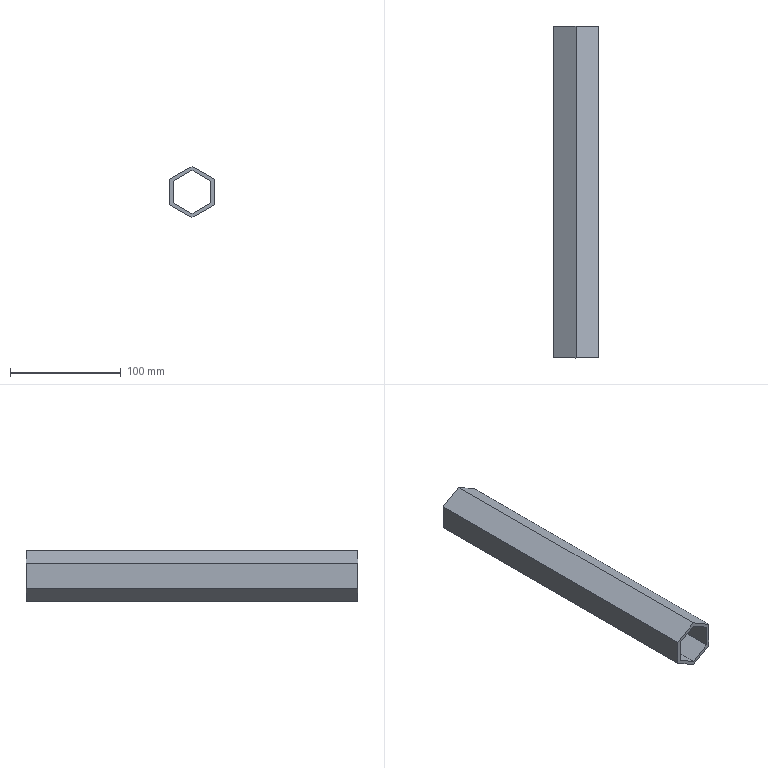Part | SolidWorks | features Extrusion 1 | 1 solid | 14 faces | box 40 x 300 x 46.188 mm | volume 115355 mm3 | plane 14
STEP:
#1=CARTESIAN_POINT('',(20.,300.,-11.547));
#2=VERTEX_POINT('',#1);
#3=CARTESIAN_POINT('',(0.,300.,-23.094));
#4=VERTEX_POINT('',#3);
#5=CARTESIAN_POINT('',(20.,300.,-11.547));
#6=DIRECTION('',(-0.866,0.,-0.5));
#7=VECTOR('',#6,1000.);
#8=LINE('',#5,#7);
#9=EDGE_CURVE('',#2,#4,#8,.T.);
#10=ORIENTED_EDGE('',*,*,#9,.T.);
#11=CARTESIAN_POINT('',(-20.,300.,-11.547));
#12=VERTEX_POINT('',#11);
#13=CARTESIAN_POINT('',(0.,300.,-23.094));
#14=DIRECTION('',(-0.866,0.,0.5));
#15=VECTOR('',#14,1000.);
#16=LINE('',#13,#15);
#17=EDGE_CURVE('',#4,#12,#16,.T.);
#18=ORIENTED_EDGE('',*,*,#17,.T.);
#19=CARTESIAN_POINT('',(-20.,300.,11.547));
#20=VERTEX_POINT('',#19);
#21=CARTESIAN_POINT('',(-20.,300.,-11.547));
#22=DIRECTION('',(0.,0.,1.));
#23=VECTOR('',#22,1000.);
#24=LINE('',#21,#23);
#25=EDGE_CURVE('',#12,#20,#24,.T.);
#26=ORIENTED_EDGE('',*,*,#25,.T.);
#27=CARTESIAN_POINT('',(0.,300.,23.094));
#28=VERTEX_POINT('',#27);
#29=CARTESIAN_POINT('',(-20.,300.,11.547));
#30=DIRECTION('',(0.866,0.,0.5));
#31=VECTOR('',#30,1000.);
#32=LINE('',#29,#31);
#33=EDGE_CURVE('',#20,#28,#32,.T.);
#34=ORIENTED_EDGE('',*,*,#33,.T.);
#35=CARTESIAN_POINT('',(20.,300.,11.547));
#36=VERTEX_POINT('',#35);
#37=CARTESIAN_POINT('',(0.,300.,23.094));
#38=DIRECTION('',(0.866,0.,-0.5));
#39=VECTOR('',#38,1000.);
#40=LINE('',#37,#39);
#41=EDGE_CURVE('',#28,#36,#40,.T.);
#42=ORIENTED_EDGE('',*,*,#41,.T.);
#43=CARTESIAN_POINT('',(20.,300.,11.547));
#44=DIRECTION('',(0.,0.,-1.));
#45=VECTOR('',#44,1000.);
#46=LINE('',#43,#45);
#47=EDGE_CURVE('',#36,#2,#46,.T.);
#48=ORIENTED_EDGE('',*,*,#47,.T.);
#49=EDGE_LOOP('',(#10,#18,#26,#34,#42,#48));
#50=FACE_OUTER_BOUND('',#49,.T.);
#51=CARTESIAN_POINT('',(-17.,300.,-9.815));
#52=VERTEX_POINT('',#51);
#53=CARTESIAN_POINT('',(-17.,300.,9.815));
#54=VERTEX_POINT('',#53);
#55=CARTESIAN_POINT('',(-17.,300.,-9.815));
#56=DIRECTION('',(0.,0.,1.));
#57=VECTOR('',#56,1000.);
#58=LINE('',#55,#57);
#59=EDGE_CURVE('',#52,#54,#58,.T.);
#60=ORIENTED_EDGE('',*,*,#59,.F.);
#61=CARTESIAN_POINT('',(0.,300.,-19.63));
#62=VERTEX_POINT('',#61);
#63=CARTESIAN_POINT('',(0.,300.,-19.63));
#64=DIRECTION('',(-0.866,0.,0.5));
#65=VECTOR('',#64,1000.);
#66=LINE('',#63,#65);
#67=EDGE_CURVE('',#62,#52,#66,.T.);
#68=ORIENTED_EDGE('',*,*,#67,.F.);
#69=CARTESIAN_POINT('',(17.,300.,-9.815));
#70=VERTEX_POINT('',#69);
#71=CARTESIAN_POINT('',(17.,300.,-9.815));
#72=DIRECTION('',(-0.866,0.,-0.5));
#73=VECTOR('',#72,1000.);
#74=LINE('',#71,#73);
#75=EDGE_CURVE('',#70,#62,#74,.T.);
#76=ORIENTED_EDGE('',*,*,#75,.F.);
#77=CARTESIAN_POINT('',(17.,300.,9.815));
#78=VERTEX_POINT('',#77);
#79=CARTESIAN_POINT('',(17.,300.,9.815));
#80=DIRECTION('',(0.,0.,-1.));
#81=VECTOR('',#80,1000.);
#82=LINE('',#79,#81);
#83=EDGE_CURVE('',#78,#70,#82,.T.);
#84=ORIENTED_EDGE('',*,*,#83,.F.);
#85=CARTESIAN_POINT('',(0.,300.,19.63));
#86=VERTEX_POINT('',#85);
#87=CARTESIAN_POINT('',(0.,300.,19.63));
#88=DIRECTION('',(0.866,0.,-0.5));
#89=VECTOR('',#88,1000.);
#90=LINE('',#87,#89);
#91=EDGE_CURVE('',#86,#78,#90,.T.);
#92=ORIENTED_EDGE('',*,*,#91,.F.);
#93=CARTESIAN_POINT('',(-17.,300.,9.815));
#94=DIRECTION('',(0.866,0.,0.5));
#95=VECTOR('',#94,1000.);
#96=LINE('',#93,#95);
#97=EDGE_CURVE('',#54,#86,#96,.T.);
#98=ORIENTED_EDGE('',*,*,#97,.F.);
#99=EDGE_LOOP('',(#60,#68,#76,#84,#92,#98));
#100=FACE_BOUND('',#99,.T.);
#101=CARTESIAN_POINT('',(0.,300.,0.));
#102=DIRECTION('',(0.,1.,0.));
#103=DIRECTION('',(0.,0.,1.));
#104=AXIS2_PLACEMENT_3D('',#101,#102,#103);
#105=PLANE('',#104);
#106=ADVANCED_FACE('',(#50,#100),#105,.T.);
#107=CARTESIAN_POINT('',(20.,0.,-11.547));
#108=VERTEX_POINT('',#107);
#109=CARTESIAN_POINT('',(0.,0.,-23.094));
#110=VERTEX_POINT('',#109);
#111=CARTESIAN_POINT('',(20.,0.,-11.547));
#112=DIRECTION('',(-0.866,0.,-0.5));
#113=VECTOR('',#112,1000.);
#114=LINE('',#111,#113);
#115=EDGE_CURVE('',#108,#110,#114,.T.);
#116=ORIENTED_EDGE('',*,*,#115,.F.);
#117=CARTESIAN_POINT('',(20.,0.,11.547));
#118=VERTEX_POINT('',#117);
#119=CARTESIAN_POINT('',(20.,0.,11.547));
#120=DIRECTION('',(0.,0.,-1.));
#121=VECTOR('',#120,1000.);
#122=LINE('',#119,#121);
#123=EDGE_CURVE('',#118,#108,#122,.T.);
#124=ORIENTED_EDGE('',*,*,#123,.F.);
#125=CARTESIAN_POINT('',(0.,0.,23.094));
#126=VERTEX_POINT('',#125);
#127=CARTESIAN_POINT('',(0.,0.,23.094));
#128=DIRECTION('',(0.866,0.,-0.5));
#129=VECTOR('',#128,1000.);
#130=LINE('',#127,#129);
#131=EDGE_CURVE('',#126,#118,#130,.T.);
#132=ORIENTED_EDGE('',*,*,#131,.F.);
#133=CARTESIAN_POINT('',(-20.,0.,11.547));
#134=VERTEX_POINT('',#133);
#135=CARTESIAN_POINT('',(-20.,0.,11.547));
#136=DIRECTION('',(0.866,0.,0.5));
#137=VECTOR('',#136,1000.);
#138=LINE('',#135,#137);
#139=EDGE_CURVE('',#134,#126,#138,.T.);
#140=ORIENTED_EDGE('',*,*,#139,.F.);
#141=CARTESIAN_POINT('',(-20.,0.,-11.547));
#142=VERTEX_POINT('',#141);
#143=CARTESIAN_POINT('',(-20.,0.,-11.547));
#144=DIRECTION('',(0.,0.,1.));
#145=VECTOR('',#144,1000.);
#146=LINE('',#143,#145);
#147=EDGE_CURVE('',#142,#134,#146,.T.);
#148=ORIENTED_EDGE('',*,*,#147,.F.);
#149=CARTESIAN_POINT('',(0.,0.,-23.094));
#150=DIRECTION('',(-0.866,0.,0.5));
#151=VECTOR('',#150,1000.);
#152=LINE('',#149,#151);
#153=EDGE_CURVE('',#110,#142,#152,.T.);
#154=ORIENTED_EDGE('',*,*,#153,.F.);
#155=EDGE_LOOP('',(#116,#124,#132,#140,#148,#154));
#156=FACE_OUTER_BOUND('',#155,.T.);
#157=CARTESIAN_POINT('',(0.,0.,-19.63));
#158=VERTEX_POINT('',#157);
#159=CARTESIAN_POINT('',(-17.,0.,-9.815));
#160=VERTEX_POINT('',#159);
#161=CARTESIAN_POINT('',(0.,0.,-19.63));
#162=DIRECTION('',(-0.866,0.,0.5));
#163=VECTOR('',#162,1000.);
#164=LINE('',#161,#163);
#165=EDGE_CURVE('',#158,#160,#164,.T.);
#166=ORIENTED_EDGE('',*,*,#165,.T.);
#167=CARTESIAN_POINT('',(-17.,0.,9.815));
#168=VERTEX_POINT('',#167);
#169=CARTESIAN_POINT('',(-17.,0.,-9.815));
#170=DIRECTION('',(0.,0.,1.));
#171=VECTOR('',#170,1000.);
#172=LINE('',#169,#171);
#173=EDGE_CURVE('',#160,#168,#172,.T.);
#174=ORIENTED_EDGE('',*,*,#173,.T.);
#175=CARTESIAN_POINT('',(0.,0.,19.63));
#176=VERTEX_POINT('',#175);
#177=CARTESIAN_POINT('',(-17.,0.,9.815));
#178=DIRECTION('',(0.866,0.,0.5));
#179=VECTOR('',#178,1000.);
#180=LINE('',#177,#179);
#181=EDGE_CURVE('',#168,#176,#180,.T.);
#182=ORIENTED_EDGE('',*,*,#181,.T.);
#183=CARTESIAN_POINT('',(17.,0.,9.815));
#184=VERTEX_POINT('',#183);
#185=CARTESIAN_POINT('',(0.,0.,19.63));
#186=DIRECTION('',(0.866,0.,-0.5));
#187=VECTOR('',#186,1000.);
#188=LINE('',#185,#187);
#189=EDGE_CURVE('',#176,#184,#188,.T.);
#190=ORIENTED_EDGE('',*,*,#189,.T.);
#191=CARTESIAN_POINT('',(17.,0.,-9.815));
#192=VERTEX_POINT('',#191);
#193=CARTESIAN_POINT('',(17.,0.,9.815));
#194=DIRECTION('',(0.,0.,-1.));
#195=VECTOR('',#194,1000.);
#196=LINE('',#193,#195);
#197=EDGE_CURVE('',#184,#192,#196,.T.);
#198=ORIENTED_EDGE('',*,*,#197,.T.);
#199=CARTESIAN_POINT('',(17.,0.,-9.815));
#200=DIRECTION('',(-0.866,0.,-0.5));
#201=VECTOR('',#200,1000.);
#202=LINE('',#199,#201);
#203=EDGE_CURVE('',#192,#158,#202,.T.);
#204=ORIENTED_EDGE('',*,*,#203,.T.);
#205=EDGE_LOOP('',(#166,#174,#182,#190,#198,#204));
#206=FACE_BOUND('',#205,.T.);
#207=CARTESIAN_POINT('',(0.,0.,0.));
#208=DIRECTION('',(0.,1.,0.));
#209=DIRECTION('',(0.,0.,1.));
#210=AXIS2_PLACEMENT_3D('',#207,#208,#209);
#211=PLANE('',#210);
#212=ADVANCED_FACE('',(#156,#206),#211,.F.);
#213=ORIENTED_EDGE('',*,*,#115,.T.);
#214=CARTESIAN_POINT('',(0.,300.,-23.094));
#215=DIRECTION('',(0.,-1.,0.));
#216=VECTOR('',#215,1000.);
#217=LINE('',#214,#216);
#218=EDGE_CURVE('',#4,#110,#217,.T.);
#219=ORIENTED_EDGE('',*,*,#218,.F.);
#220=ORIENTED_EDGE('',*,*,#9,.F.);
#221=CARTESIAN_POINT('',(20.,300.,-11.547));
#222=DIRECTION('',(0.,-1.,0.));
#223=VECTOR('',#222,1000.);
#224=LINE('',#221,#223);
#225=EDGE_CURVE('',#2,#108,#224,.T.);
#226=ORIENTED_EDGE('',*,*,#225,.T.);
#227=EDGE_LOOP('',(#213,#219,#220,#226));
#228=FACE_OUTER_BOUND('',#227,.T.);
#229=CARTESIAN_POINT('',(20.,300.,-11.547));
#230=DIRECTION('',(-0.5,0.,0.866));
#231=DIRECTION('',(0.866,0.,0.5));
#232=AXIS2_PLACEMENT_3D('',#229,#230,#231);
#233=PLANE('',#232);
#234=ADVANCED_FACE('',(#228),#233,.F.);
#235=ORIENTED_EDGE('',*,*,#153,.T.);
#236=CARTESIAN_POINT('',(-20.,300.,-11.547));
#237=DIRECTION('',(0.,-1.,0.));
#238=VECTOR('',#237,1000.);
#239=LINE('',#236,#238);
#240=EDGE_CURVE('',#12,#142,#239,.T.);
#241=ORIENTED_EDGE('',*,*,#240,.F.);
#242=ORIENTED_EDGE('',*,*,#17,.F.);
#243=ORIENTED_EDGE('',*,*,#218,.T.);
#244=EDGE_LOOP('',(#235,#241,#242,#243));
#245=FACE_OUTER_BOUND('',#244,.T.);
#246=CARTESIAN_POINT('',(0.,300.,-23.094));
#247=DIRECTION('',(0.5,0.,0.866));
#248=DIRECTION('',(0.866,0.,-0.5));
#249=AXIS2_PLACEMENT_3D('',#246,#247,#248);
#250=PLANE('',#249);
#251=ADVANCED_FACE('',(#245),#250,.F.);
#252=ORIENTED_EDGE('',*,*,#147,.T.);
#253=CARTESIAN_POINT('',(-20.,300.,11.547));
#254=DIRECTION('',(0.,-1.,0.));
#255=VECTOR('',#254,1000.);
#256=LINE('',#253,#255);
#257=EDGE_CURVE('',#20,#134,#256,.T.);
#258=ORIENTED_EDGE('',*,*,#257,.F.);
#259=ORIENTED_EDGE('',*,*,#25,.F.);
#260=ORIENTED_EDGE('',*,*,#240,.T.);
#261=EDGE_LOOP('',(#252,#258,#259,#260));
#262=FACE_OUTER_BOUND('',#261,.T.);
#263=CARTESIAN_POINT('',(-20.,300.,-11.547));
#264=DIRECTION('',(1.,0.,0.));
#265=DIRECTION('',(0.,0.,-1.));
#266=AXIS2_PLACEMENT_3D('',#263,#264,#265);
#267=PLANE('',#266);
#268=ADVANCED_FACE('',(#262),#267,.F.);
#269=ORIENTED_EDGE('',*,*,#139,.T.);
#270=CARTESIAN_POINT('',(0.,300.,23.094));
#271=DIRECTION('',(0.,-1.,0.));
#272=VECTOR('',#271,1000.);
#273=LINE('',#270,#272);
#274=EDGE_CURVE('',#28,#126,#273,.T.);
#275=ORIENTED_EDGE('',*,*,#274,.F.);
#276=ORIENTED_EDGE('',*,*,#33,.F.);
#277=ORIENTED_EDGE('',*,*,#257,.T.);
#278=EDGE_LOOP('',(#269,#275,#276,#277));
#279=FACE_OUTER_BOUND('',#278,.T.);
#280=CARTESIAN_POINT('',(-20.,300.,11.547));
#281=DIRECTION('',(0.5,0.,-0.866));
#282=DIRECTION('',(-0.866,0.,-0.5));
#283=AXIS2_PLACEMENT_3D('',#280,#281,#282);
#284=PLANE('',#283);
#285=ADVANCED_FACE('',(#279),#284,.F.);
#286=ORIENTED_EDGE('',*,*,#131,.T.);
#287=CARTESIAN_POINT('',(20.,300.,11.547));
#288=DIRECTION('',(0.,-1.,0.));
#289=VECTOR('',#288,1000.);
#290=LINE('',#287,#289);
#291=EDGE_CURVE('',#36,#118,#290,.T.);
#292=ORIENTED_EDGE('',*,*,#291,.F.);
#293=ORIENTED_EDGE('',*,*,#41,.F.);
#294=ORIENTED_EDGE('',*,*,#274,.T.);
#295=EDGE_LOOP('',(#286,#292,#293,#294));
#296=FACE_OUTER_BOUND('',#295,.T.);
#297=CARTESIAN_POINT('',(0.,300.,23.094));
#298=DIRECTION('',(-0.5,0.,-0.866));
#299=DIRECTION('',(-0.866,0.,0.5));
#300=AXIS2_PLACEMENT_3D('',#297,#298,#299);
#301=PLANE('',#300);
#302=ADVANCED_FACE('',(#296),#301,.F.);
#303=ORIENTED_EDGE('',*,*,#123,.T.);
#304=ORIENTED_EDGE('',*,*,#225,.F.);
#305=ORIENTED_EDGE('',*,*,#47,.F.);
#306=ORIENTED_EDGE('',*,*,#291,.T.);
#307=EDGE_LOOP('',(#303,#304,#305,#306));
#308=FACE_OUTER_BOUND('',#307,.T.);
#309=CARTESIAN_POINT('',(20.,300.,11.547));
#310=DIRECTION('',(-1.,0.,0.));
#311=DIRECTION('',(0.,0.,1.));
#312=AXIS2_PLACEMENT_3D('',#309,#310,#311);
#313=PLANE('',#312);
#314=ADVANCED_FACE('',(#308),#313,.F.);
#315=ORIENTED_EDGE('',*,*,#165,.F.);
#316=CARTESIAN_POINT('',(0.,300.,-19.63));
#317=DIRECTION('',(0.,-1.,0.));
#318=VECTOR('',#317,1000.);
#319=LINE('',#316,#318);
#320=EDGE_CURVE('',#62,#158,#319,.T.);
#321=ORIENTED_EDGE('',*,*,#320,.F.);
#322=ORIENTED_EDGE('',*,*,#67,.T.);
#323=CARTESIAN_POINT('',(-17.,300.,-9.815));
#324=DIRECTION('',(0.,-1.,0.));
#325=VECTOR('',#324,1000.);
#326=LINE('',#323,#325);
#327=EDGE_CURVE('',#52,#160,#326,.T.);
#328=ORIENTED_EDGE('',*,*,#327,.T.);
#329=EDGE_LOOP('',(#315,#321,#322,#328));
#330=FACE_OUTER_BOUND('',#329,.T.);
#331=CARTESIAN_POINT('',(0.,300.,-19.63));
#332=DIRECTION('',(0.5,0.,0.866));
#333=DIRECTION('',(0.866,0.,-0.5));
#334=AXIS2_PLACEMENT_3D('',#331,#332,#333);
#335=PLANE('',#334);
#336=ADVANCED_FACE('',(#330),#335,.T.);
#337=ORIENTED_EDGE('',*,*,#173,.F.);
#338=ORIENTED_EDGE('',*,*,#327,.F.);
#339=ORIENTED_EDGE('',*,*,#59,.T.);
#340=CARTESIAN_POINT('',(-17.,300.,9.815));
#341=DIRECTION('',(0.,-1.,0.));
#342=VECTOR('',#341,1000.);
#343=LINE('',#340,#342);
#344=EDGE_CURVE('',#54,#168,#343,.T.);
#345=ORIENTED_EDGE('',*,*,#344,.T.);
#346=EDGE_LOOP('',(#337,#338,#339,#345));
#347=FACE_OUTER_BOUND('',#346,.T.);
#348=CARTESIAN_POINT('',(-17.,300.,-9.815));
#349=DIRECTION('',(1.,0.,0.));
#350=DIRECTION('',(0.,0.,-1.));
#351=AXIS2_PLACEMENT_3D('',#348,#349,#350);
#352=PLANE('',#351);
#353=ADVANCED_FACE('',(#347),#352,.T.);
#354=ORIENTED_EDGE('',*,*,#181,.F.);
#355=ORIENTED_EDGE('',*,*,#344,.F.);
#356=ORIENTED_EDGE('',*,*,#97,.T.);
#357=CARTESIAN_POINT('',(0.,300.,19.63));
#358=DIRECTION('',(0.,-1.,0.));
#359=VECTOR('',#358,1000.);
#360=LINE('',#357,#359);
#361=EDGE_CURVE('',#86,#176,#360,.T.);
#362=ORIENTED_EDGE('',*,*,#361,.T.);
#363=EDGE_LOOP('',(#354,#355,#356,#362));
#364=FACE_OUTER_BOUND('',#363,.T.);
#365=CARTESIAN_POINT('',(-17.,300.,9.815));
#366=DIRECTION('',(0.5,0.,-0.866));
#367=DIRECTION('',(-0.866,0.,-0.5));
#368=AXIS2_PLACEMENT_3D('',#365,#366,#367);
#369=PLANE('',#368);
#370=ADVANCED_FACE('',(#364),#369,.T.);
#371=ORIENTED_EDGE('',*,*,#189,.F.);
#372=ORIENTED_EDGE('',*,*,#361,.F.);
#373=ORIENTED_EDGE('',*,*,#91,.T.);
#374=CARTESIAN_POINT('',(17.,300.,9.815));
#375=DIRECTION('',(0.,-1.,0.));
#376=VECTOR('',#375,1000.);
#377=LINE('',#374,#376);
#378=EDGE_CURVE('',#78,#184,#377,.T.);
#379=ORIENTED_EDGE('',*,*,#378,.T.);
#380=EDGE_LOOP('',(#371,#372,#373,#379));
#381=FACE_OUTER_BOUND('',#380,.T.);
#382=CARTESIAN_POINT('',(0.,300.,19.63));
#383=DIRECTION('',(-0.5,0.,-0.866));
#384=DIRECTION('',(-0.866,0.,0.5));
#385=AXIS2_PLACEMENT_3D('',#382,#383,#384);
#386=PLANE('',#385);
#387=ADVANCED_FACE('',(#381),#386,.T.);
#388=ORIENTED_EDGE('',*,*,#197,.F.);
#389=ORIENTED_EDGE('',*,*,#378,.F.);
#390=ORIENTED_EDGE('',*,*,#83,.T.);
#391=CARTESIAN_POINT('',(17.,300.,-9.815));
#392=DIRECTION('',(0.,-1.,0.));
#393=VECTOR('',#392,1000.);
#394=LINE('',#391,#393);
#395=EDGE_CURVE('',#70,#192,#394,.T.);
#396=ORIENTED_EDGE('',*,*,#395,.T.);
#397=EDGE_LOOP('',(#388,#389,#390,#396));
#398=FACE_OUTER_BOUND('',#397,.T.);
#399=CARTESIAN_POINT('',(17.,300.,9.815));
#400=DIRECTION('',(-1.,0.,0.));
#401=DIRECTION('',(0.,0.,1.));
#402=AXIS2_PLACEMENT_3D('',#399,#400,#401);
#403=PLANE('',#402);
#404=ADVANCED_FACE('',(#398),#403,.T.);
#405=ORIENTED_EDGE('',*,*,#203,.F.);
#406=ORIENTED_EDGE('',*,*,#395,.F.);
#407=ORIENTED_EDGE('',*,*,#75,.T.);
#408=ORIENTED_EDGE('',*,*,#320,.T.);
#409=EDGE_LOOP('',(#405,#406,#407,#408));
#410=FACE_OUTER_BOUND('',#409,.T.);
#411=CARTESIAN_POINT('',(17.,300.,-9.815));
#412=DIRECTION('',(-0.5,0.,0.866));
#413=DIRECTION('',(0.866,0.,0.5));
#414=AXIS2_PLACEMENT_3D('',#411,#412,#413);
#415=PLANE('',#414);
#416=ADVANCED_FACE('',(#410),#415,.T.);
#417=CLOSED_SHELL('',(#106,#212,#234,#251,#268,#285,#302,#314,#336,#353,#370,#387,#404,#416));
#418=MANIFOLD_SOLID_BREP('',#417);
#419=CARTESIAN_POINT('',(0.,0.,0.));
#420=DIRECTION('',(0.,0.,1.));
#421=DIRECTION('',(1.,0.,0.));
#422=AXIS2_PLACEMENT_3D('',#419,#420,#421);
#423=(LENGTH_UNIT()NAMED_UNIT(*)SI_UNIT(.MILLI.,.METRE.));
#424=UNCERTAINTY_MEASURE_WITH_UNIT(LENGTH_MEASURE(0.00001),#423,'','');
#425=(NAMED_UNIT(*)PLANE_ANGLE_UNIT()SI_UNIT($,.RADIAN.));
#426=(NAMED_UNIT(*)SI_UNIT($,.STERADIAN.)SOLID_ANGLE_UNIT());
#427=(GEOMETRIC_REPRESENTATION_CONTEXT(3)GLOBAL_UNCERTAINTY_ASSIGNED_CONTEXT((#424))GLOBAL_UNIT_ASSIGNED_CONTEXT((#423,#425,#426))REPRESENTATION_CONTEXT('',''));
#428=ADVANCED_BREP_SHAPE_REPRESENTATION('',(#418,#422),#427);